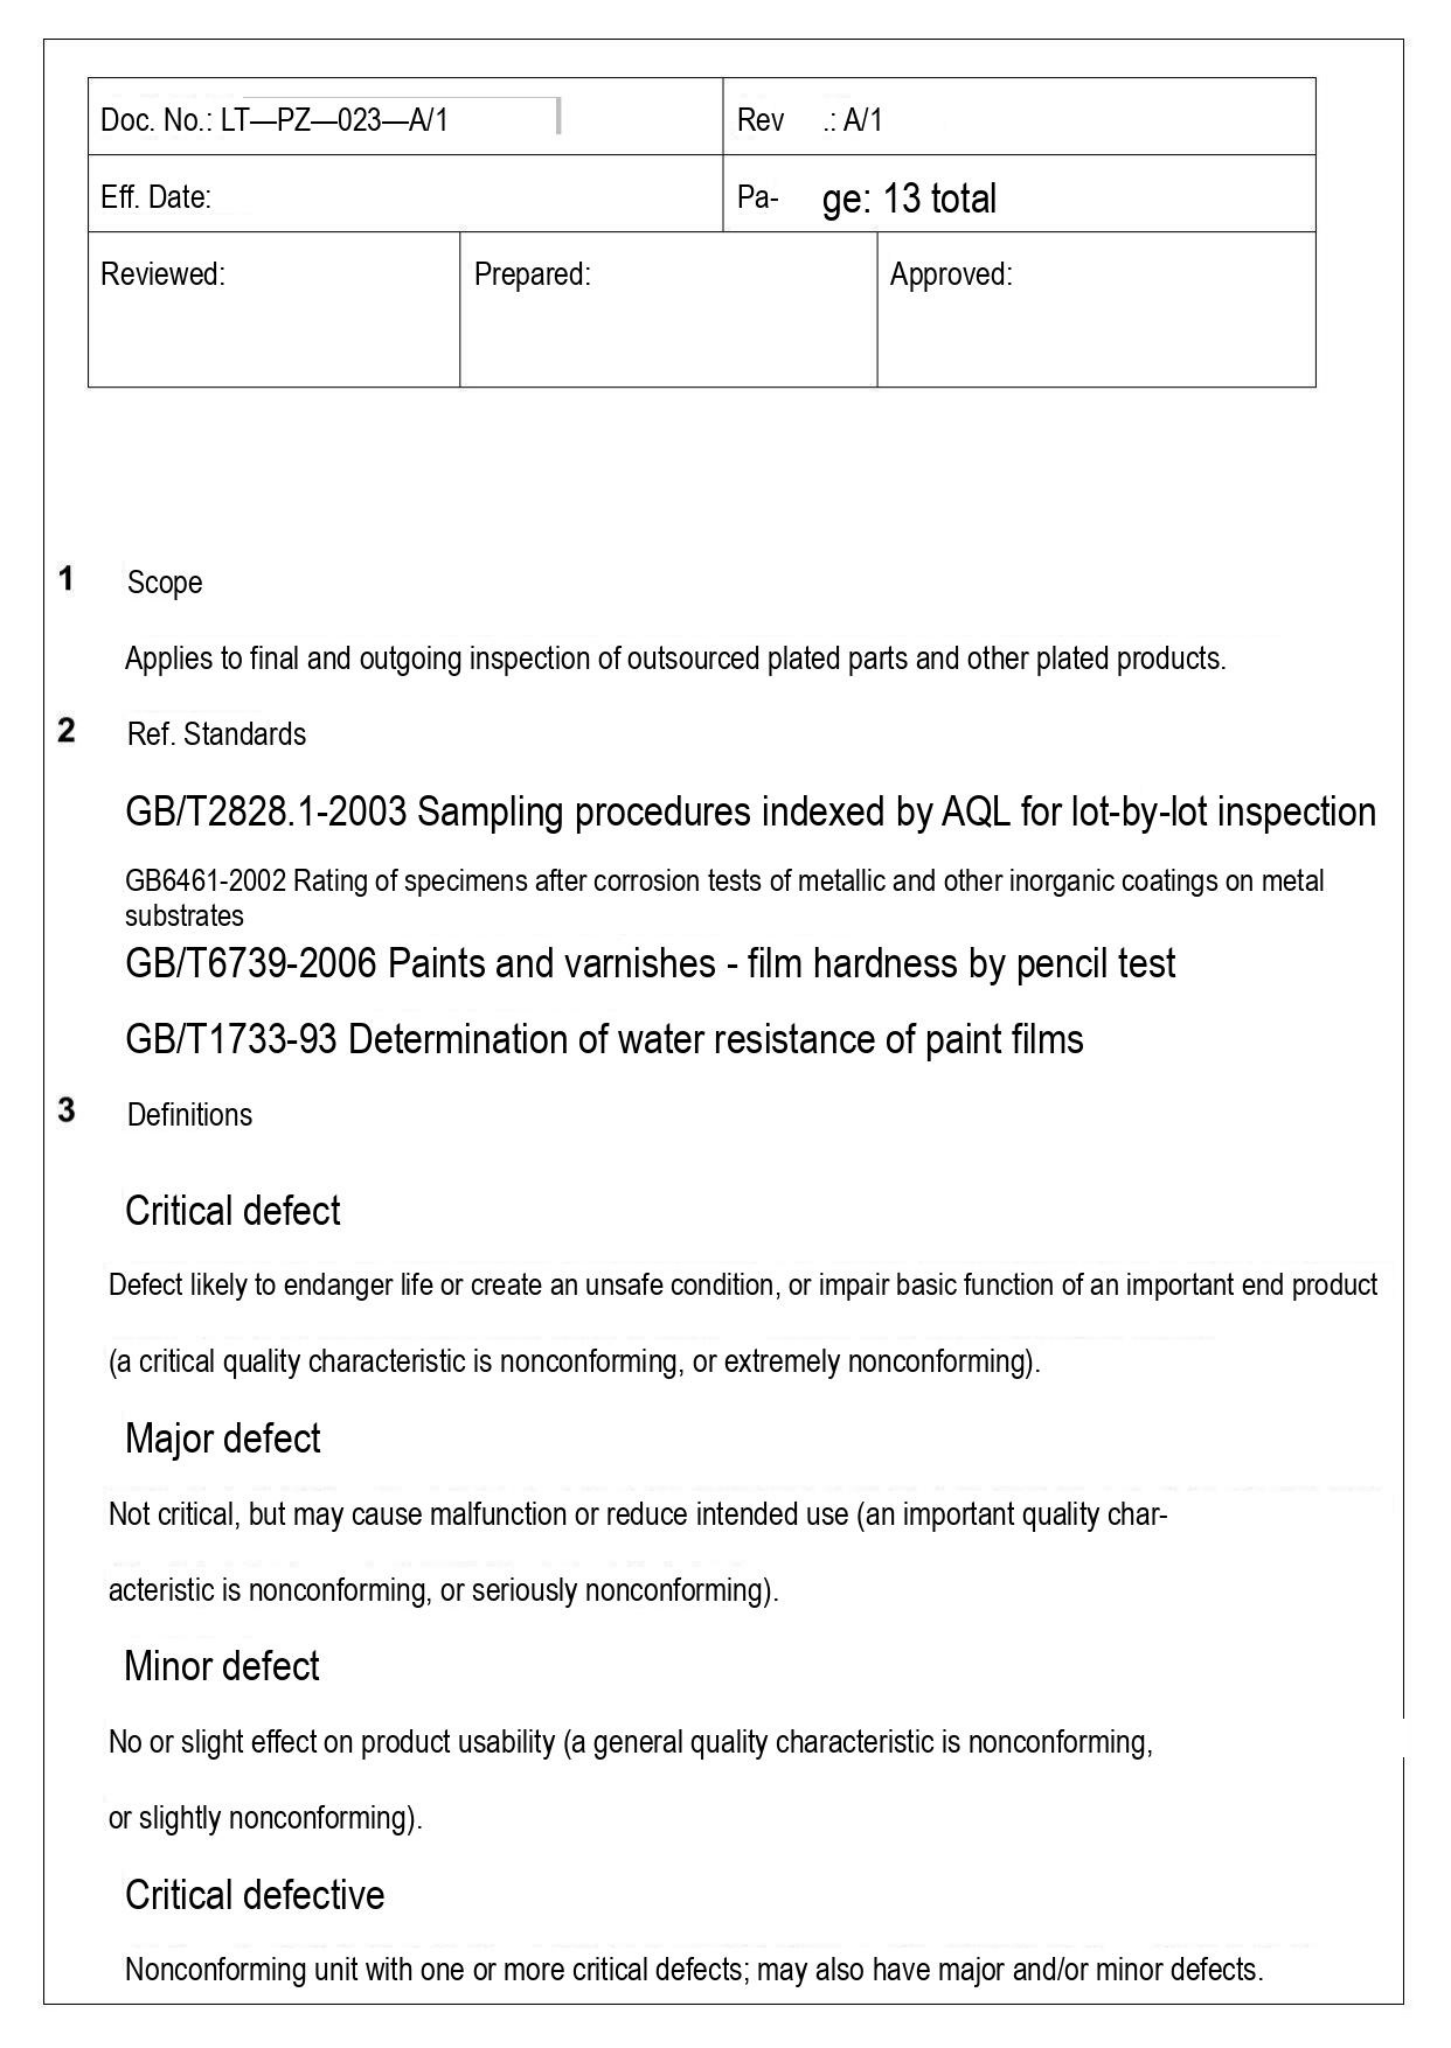| Doc. No.: LT—PZ—023—A/1 | | Rev .: A/1 |
|---|---|---|
| Eff. Date: | | Pa- ge: 13 total |
| Reviewed: | Prepared: | Approved: |

1 Scope

Applies to final and outgoing inspection of outsourced plated parts and other plated products.

2 Ref. Standards

GB/T2828.1-2003 Sampling procedures indexed by AQL for lot-by-lot inspection

GB6461-2002 Rating of specimens after corrosion tests of metallic and other inorganic coatings on metal substrates

GB/T6739-2006 Paints and varnishes - film hardness by pencil test

GB/T1733-93 Determination of water resistance of paint films

3 Definitions

Critical defect

Defect likely to endanger life or create an unsafe condition, or impair basic function of an important end product

(a critical quality characteristic is nonconforming, or extremely nonconforming).

Major defect

Not critical, but may cause malfunction or reduce intended use (an important quality char-

acteristic is nonconforming, or seriously nonconforming).

Minor defect

No or slight effect on product usability (a general quality characteristic is nonconforming,

or slightly nonconforming).

Critical defective

Nonconforming unit with one or more critical defects; may also have major and/or minor defects.
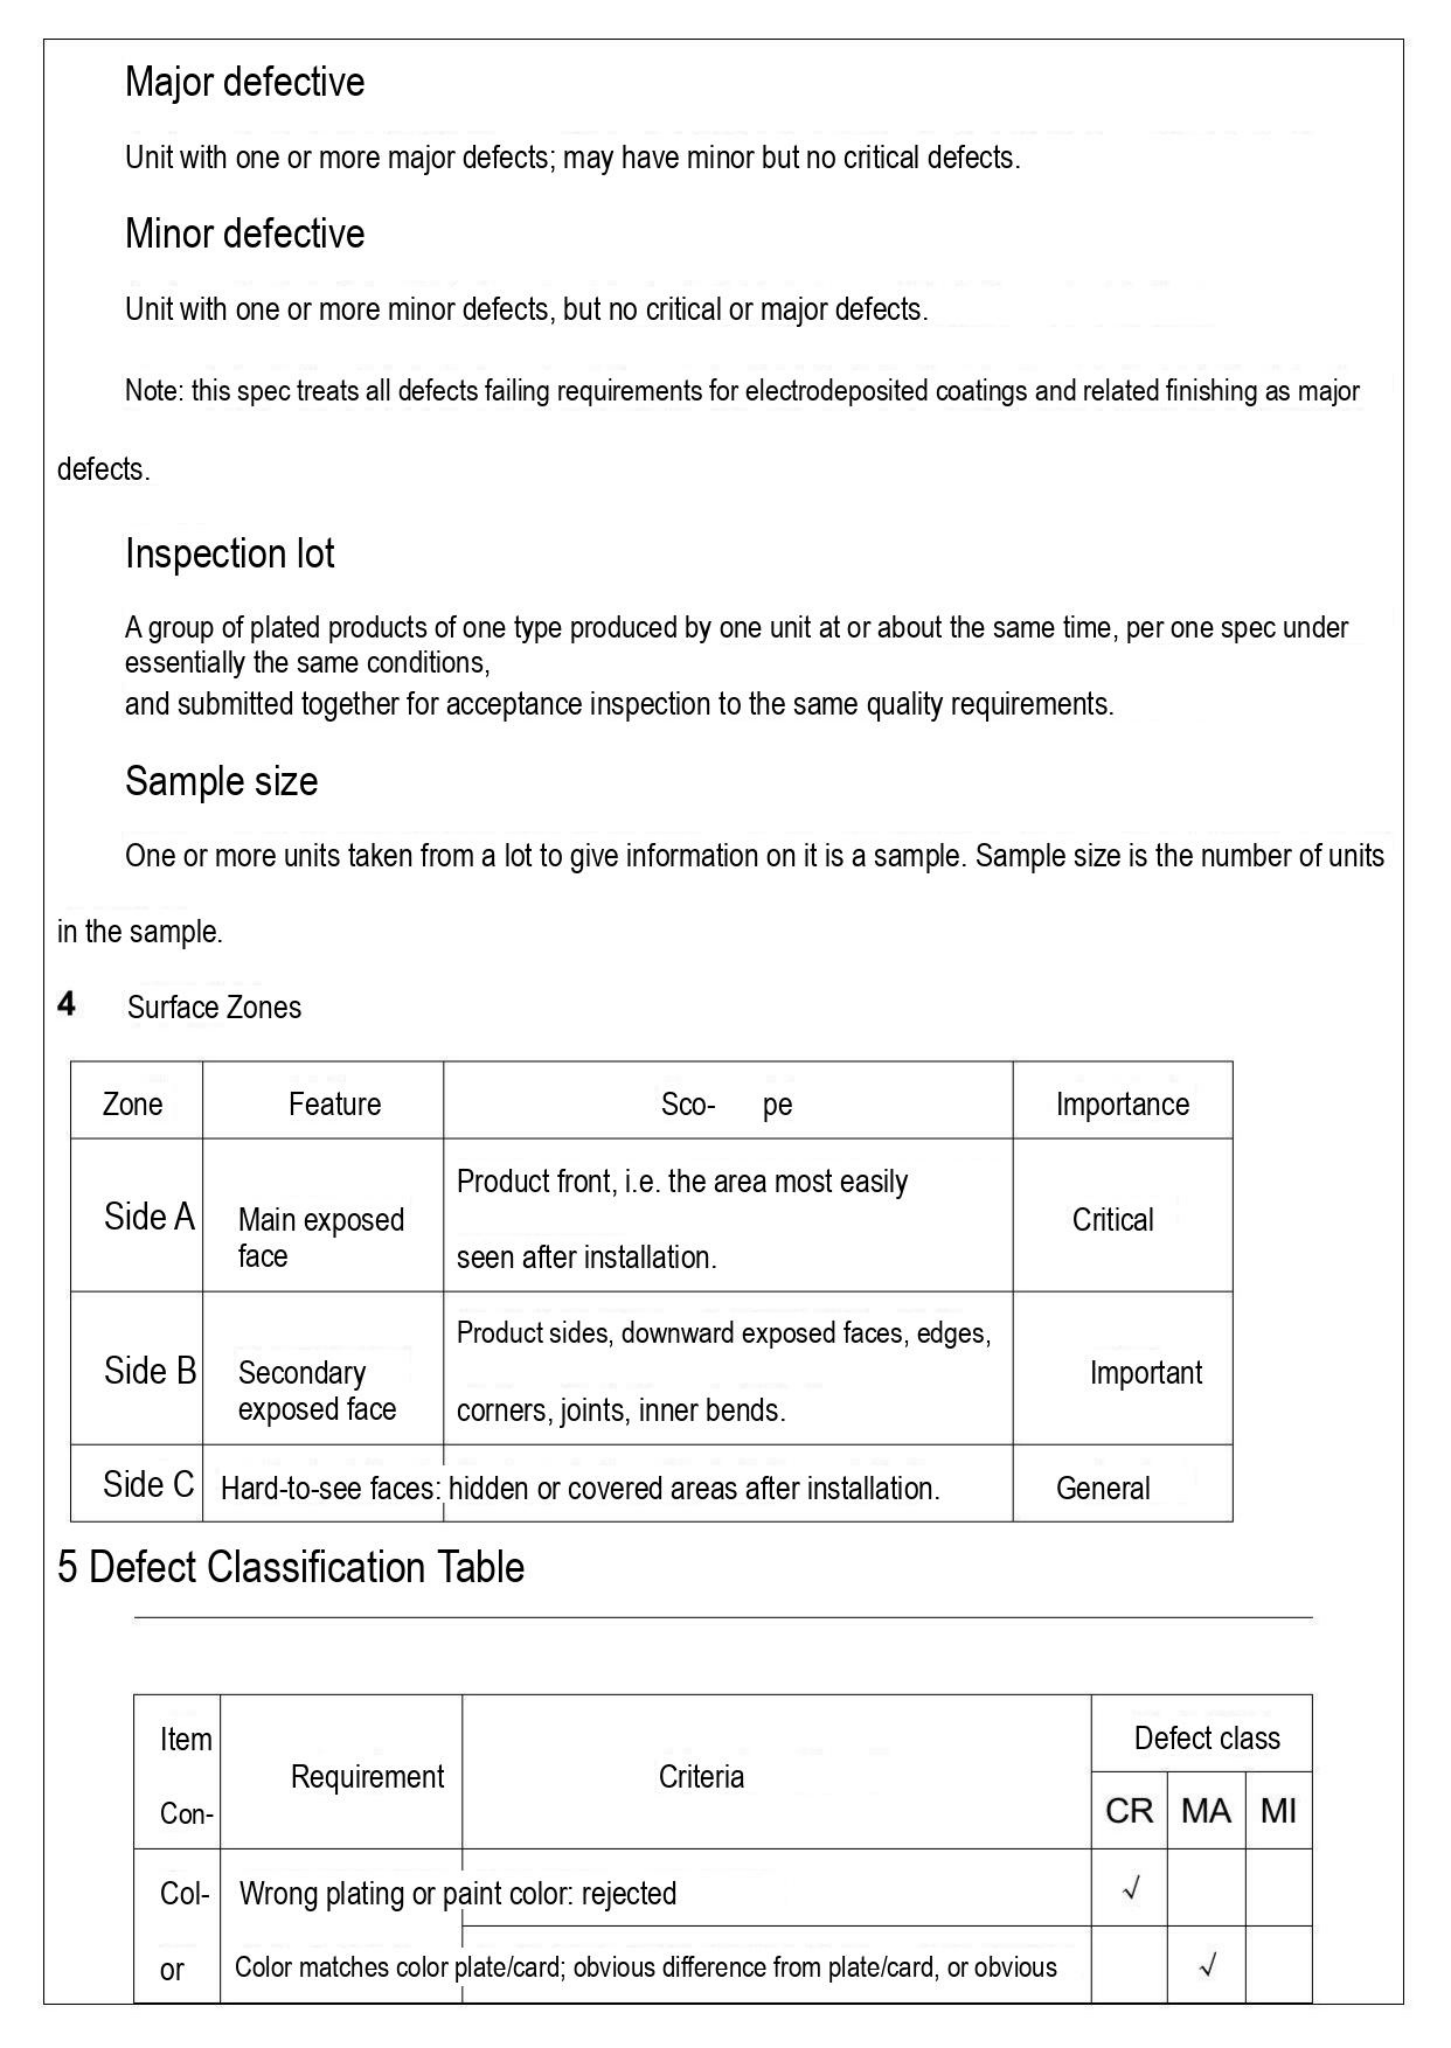Major defective

Unit with one or more major defects; may have minor but no critical defects.

Minor defective

Unit with one or more minor defects, but no critical or major defects.

Note: this spec treats all defects failing requirements for electrodeposited coatings and related finishing as major defects.

Inspection lot

A group of plated products of one type produced by one unit at or about the same time, per one spec under essentially the same conditions,
and submitted together for acceptance inspection to the same quality requirements.

Sample size

One or more units taken from a lot to give information on it is a sample. Sample size is the number of units in the sample.

4 Surface Zones

| Zone | Feature | Sco- pe | Importance |
|---|---|---|---|
| Side A | Main exposed face | Product front, i.e. the area most easily seen after installation. | Critical |
| Side B | Secondary exposed face | Product sides, downward exposed faces, edges, corners, joints, inner bends. | Important |
| Side C | Hard-to-see faces: hidden or covered areas after installation. | | General |

5 Defect Classification Table

| Item Con- | Requirement | Criteria | Defect class CR | Defect class MA | Defect class MI |
|---|---|---|---|---|---|
| Col- or | Wrong plating or paint color: rejected | | √ | | |
| | Color matches color plate/card; obvious difference from plate/card, or obvious | | | √ | |
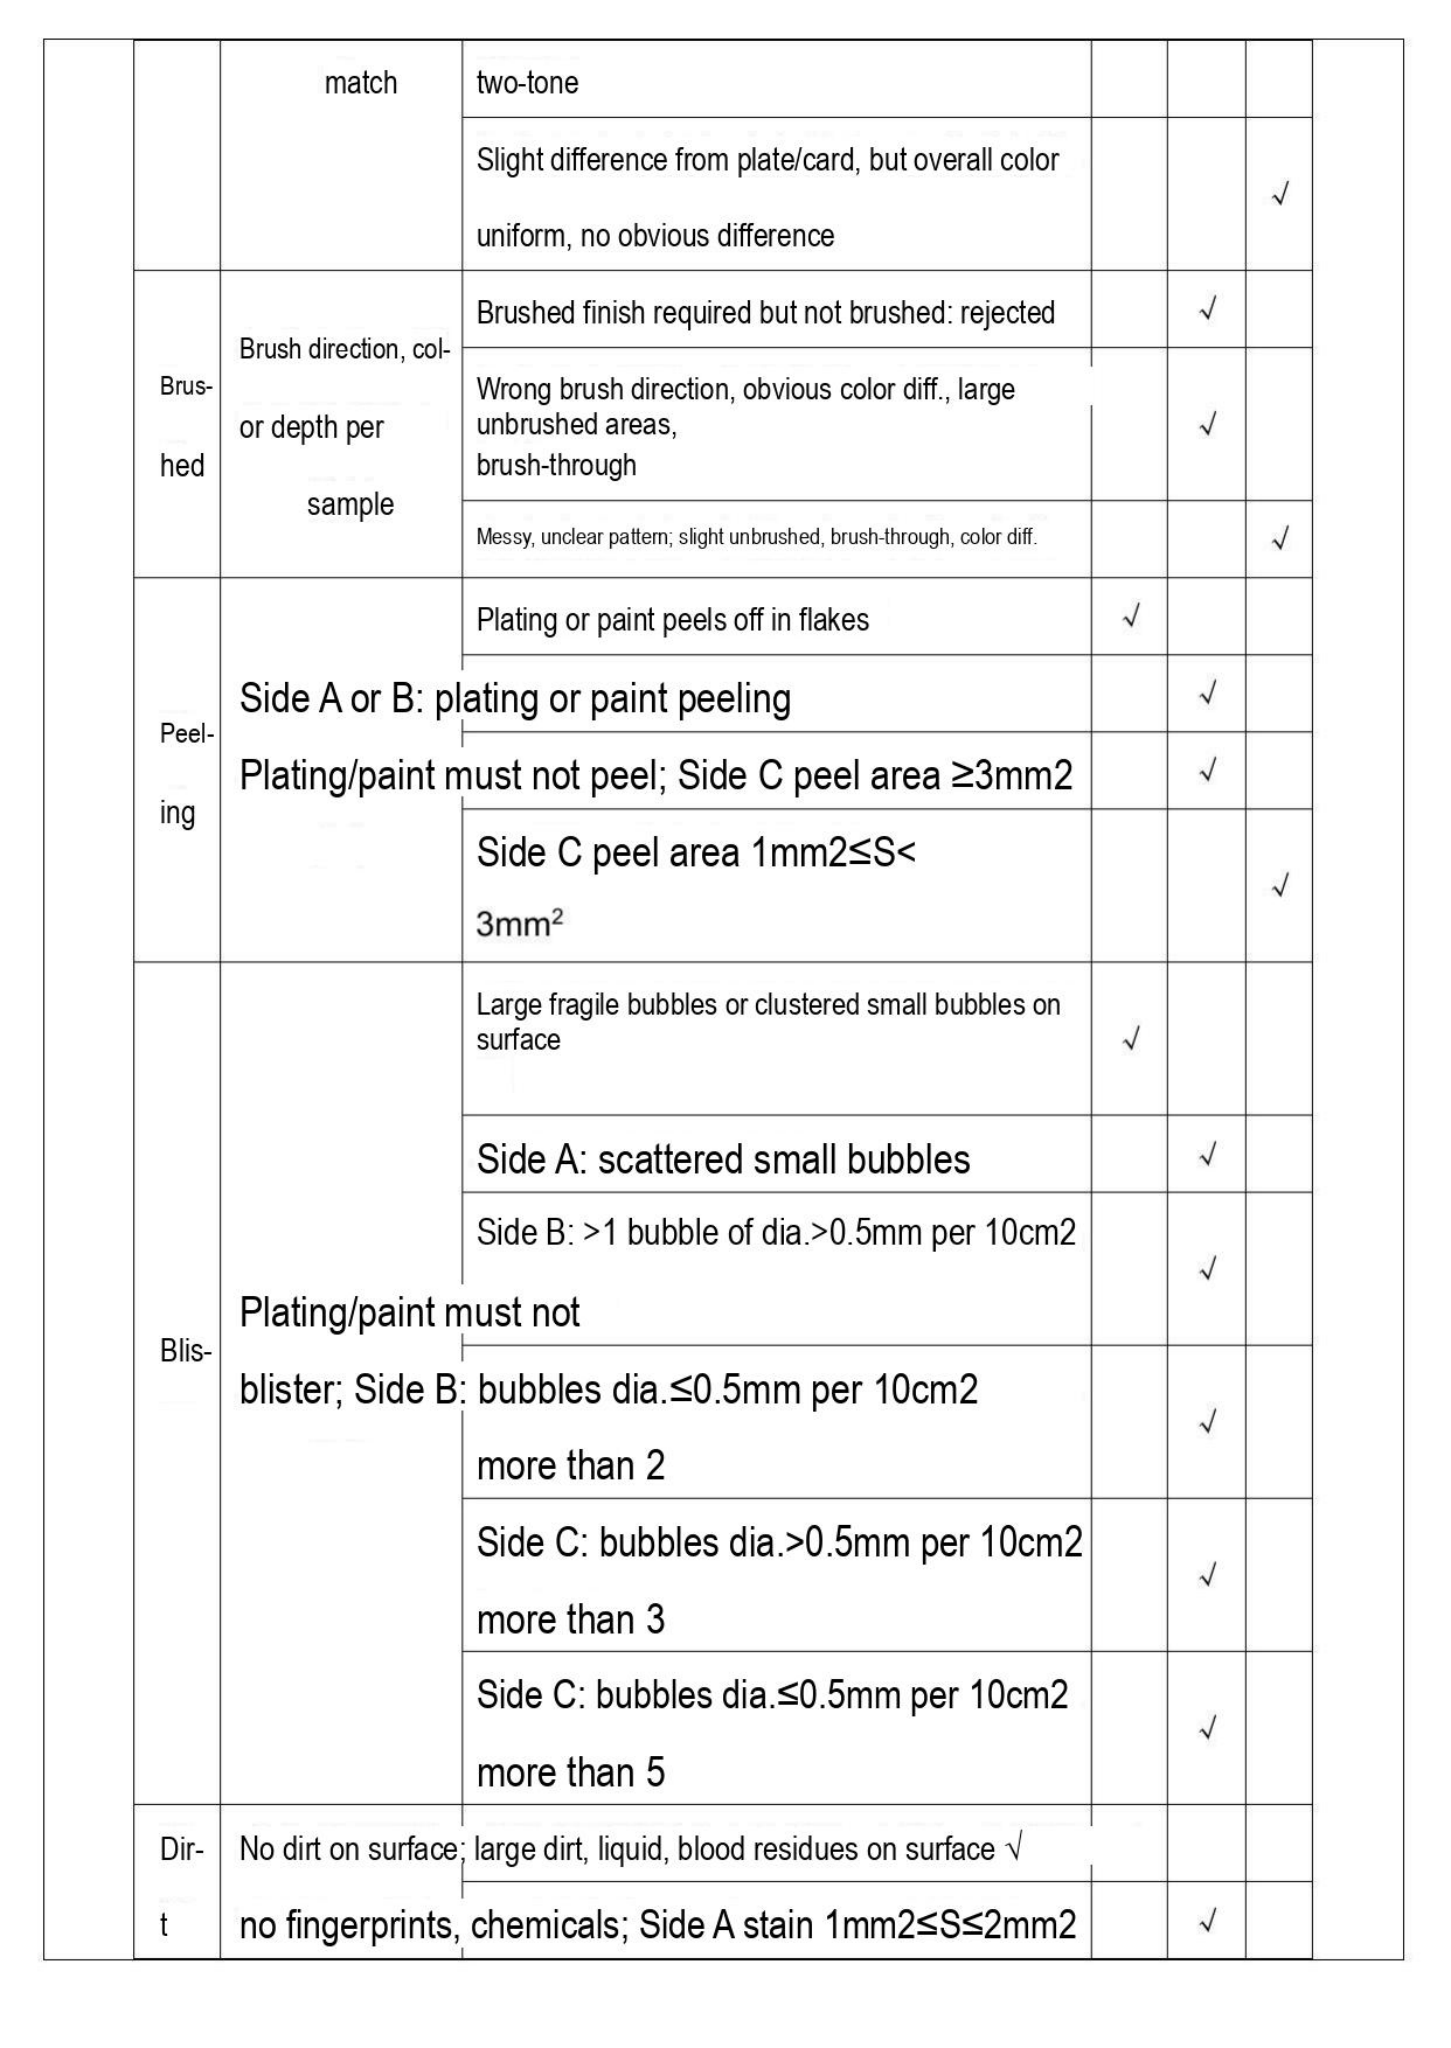| | | | | | | | |
|---|---|---|---|---|---|---|---|
| | | match | two-tone | | | | |
| | | | Slight difference from plate/card, but overall color uniform, no obvious difference | | | √ | |
| | Brus- hed | Brush direction, col- or depth per sample | Brushed finish required but not brushed: rejected | | √ | | |
| | | | Wrong brush direction, obvious color diff., large unbrushed areas, brush-through | | √ | | |
| | | | Messy, unclear pattern; slight unbrushed, brush-through, color diff. | | | √ | |
| | Peel- ing | | Plating or paint peels off in flakes | √ | | | |
| | | | Side A or B: plating or paint peeling | | √ | | |
| | | Plating/paint must not peel; | Side C peel area ≥3mm2 | | √ | | |
| | | | Side C peel area 1mm2≤S< 3mm² | | | √ | |
| | Blis- | | Large fragile bubbles or clustered small bubbles on surface | √ | | | |
| | | | Side A: scattered small bubbles | | √ | | |
| | | | Side B: >1 bubble of dia.>0.5mm per 10cm2 | | √ | | |
| | | Plating/paint must not blister; | Side B: bubbles dia.≤0.5mm per 10cm2 more than 2 | | √ | | |
| | | | Side C: bubbles dia.>0.5mm per 10cm2 more than 3 | | √ | | |
| | | | Side C: bubbles dia.≤0.5mm per 10cm2 more than 5 | | √ | | |
| | Dir- t | No dirt on surface; | large dirt, liquid, blood residues on surface √ | | | | |
| | | no fingerprints, chemicals; | Side A stain 1mm2≤S≤2mm2 | | √ | | |
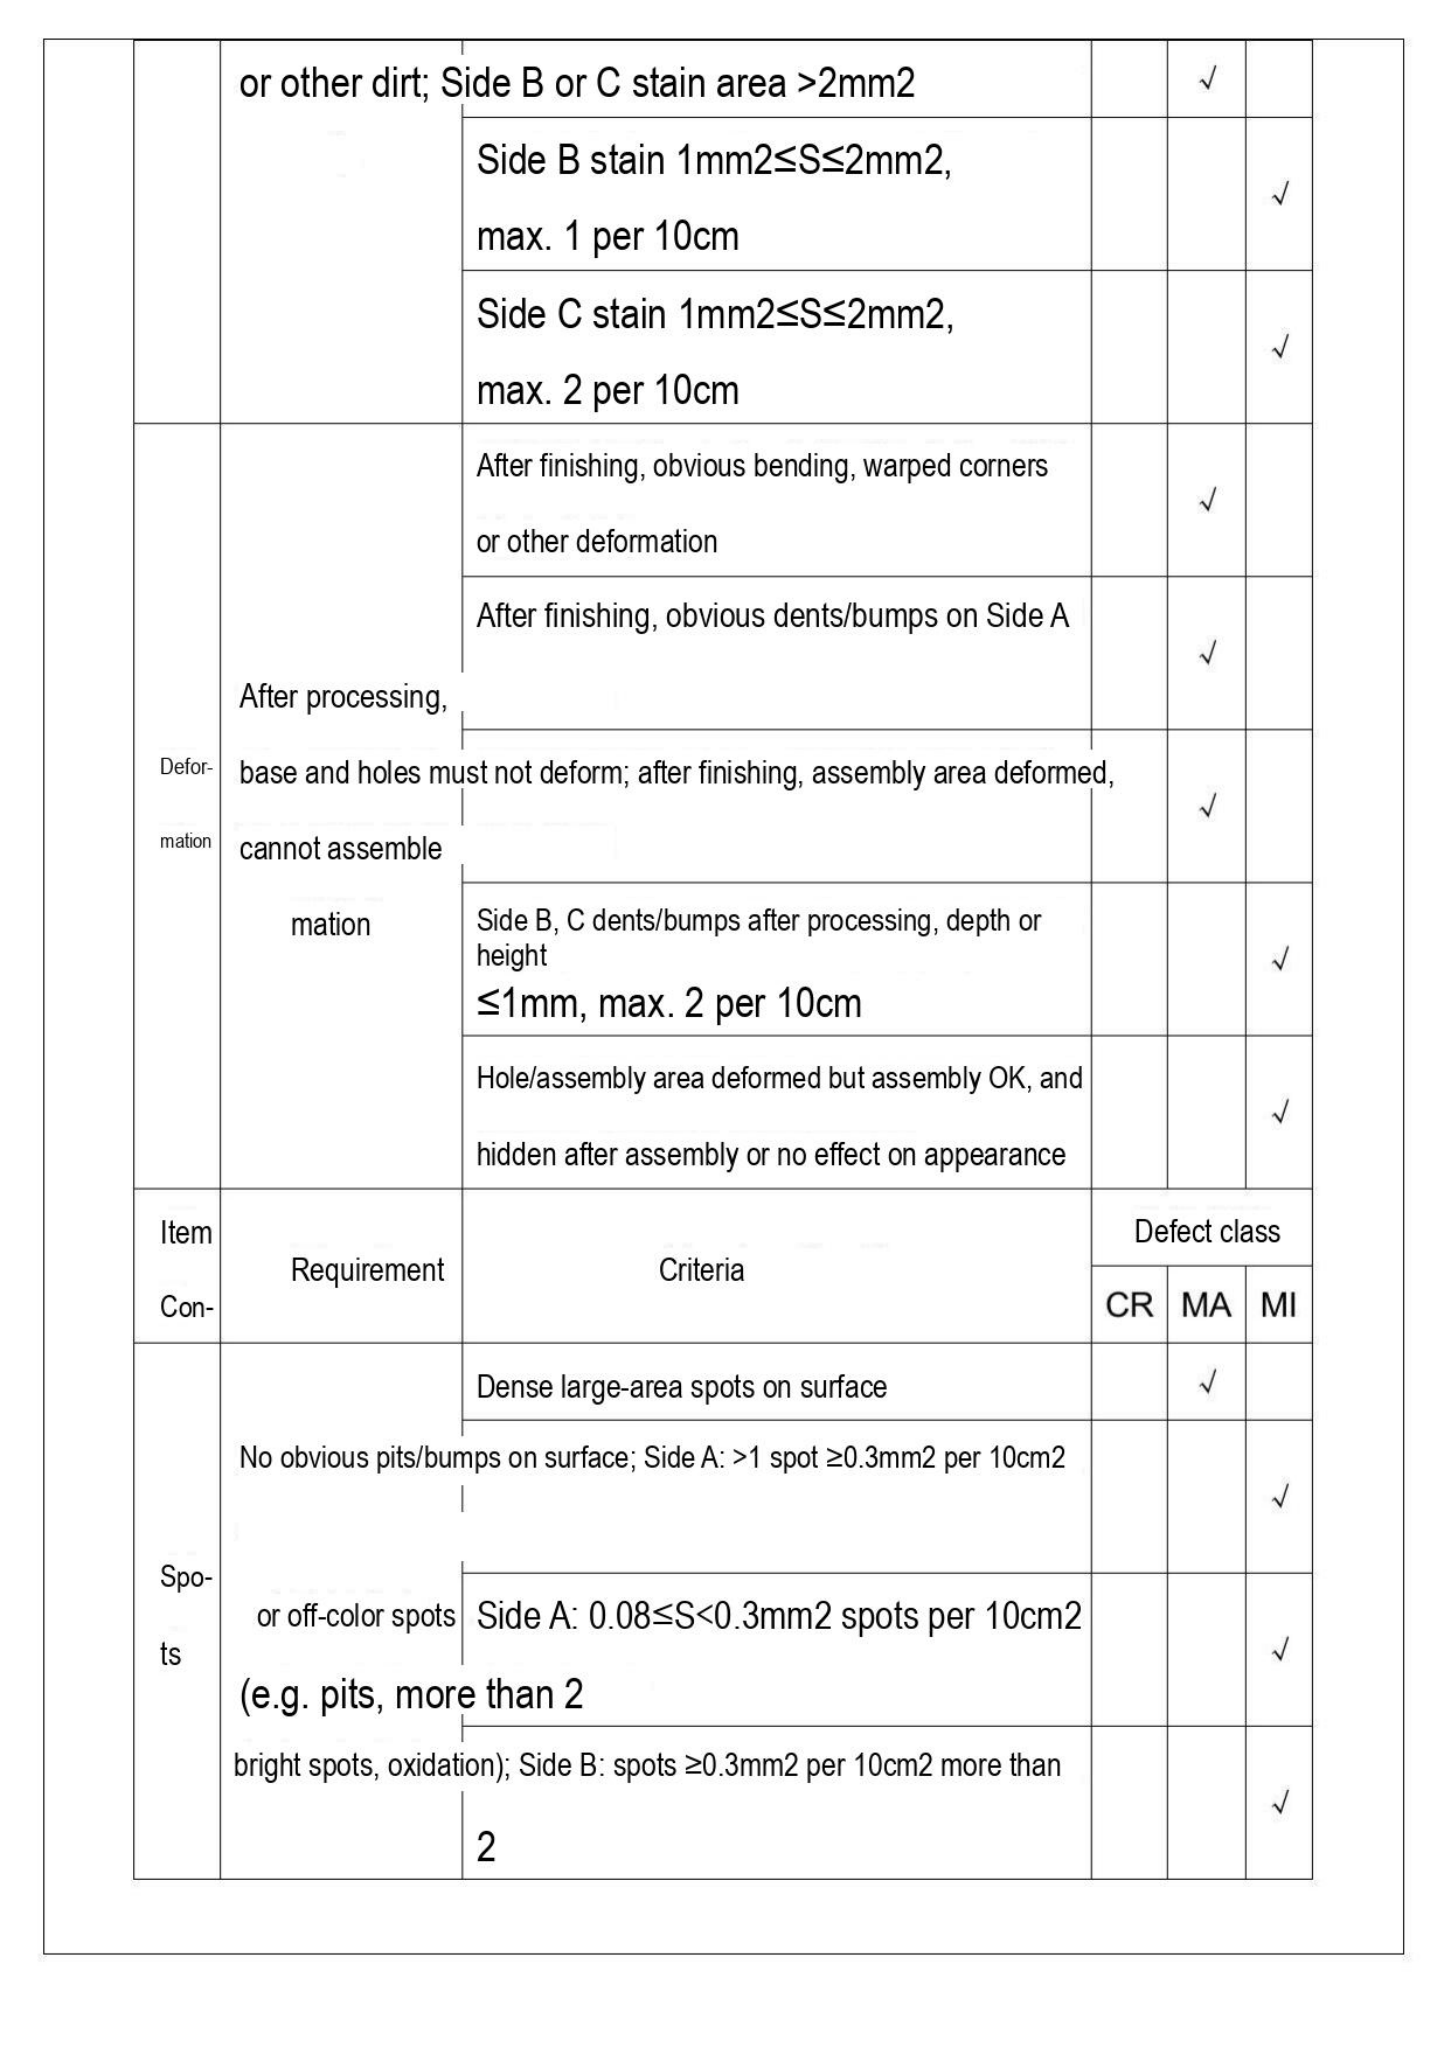| | | | | | |
|---|---|---|---|---|---|
| | or other dirt; Side B or C stain area >2mm2 | | | √ | |
| | | Side B stain 1mm2≤S≤2mm2, max. 1 per 10cm | | | √ |
| | | Side C stain 1mm2≤S≤2mm2, max. 2 per 10cm | | | √ |
| Defor- mation | | After finishing, obvious bending, warped corners or other deformation | | √ | |
| | | After finishing, obvious dents/bumps on Side A | | √ | |
| | After processing, base and holes must not deform; after finishing, assembly area deformed, cannot assemble | | | √ | |
| | mation | Side B, C dents/bumps after processing, depth or height ≤1mm, max. 2 per 10cm | | | √ |
| | | Hole/assembly area deformed but assembly OK, and hidden after assembly or no effect on appearance | | | √ |

| Item Con- | Requirement | Criteria | Defect class CR | Defect class MA | Defect class MI |
|---|---|---|---|---|---|
| Spo- ts | | Dense large-area spots on surface | | √ | |
| | No obvious pits/bumps on surface; Side A: >1 spot ≥0.3mm2 per 10cm2 | | | | √ |
| | or off-color spots (e.g. pits, more than 2 | Side A: 0.08≤S<0.3mm2 spots per 10cm2 | | | √ |
| | bright spots, oxidation); Side B: spots ≥0.3mm2 per 10cm2 more than 2 | | | | √ |
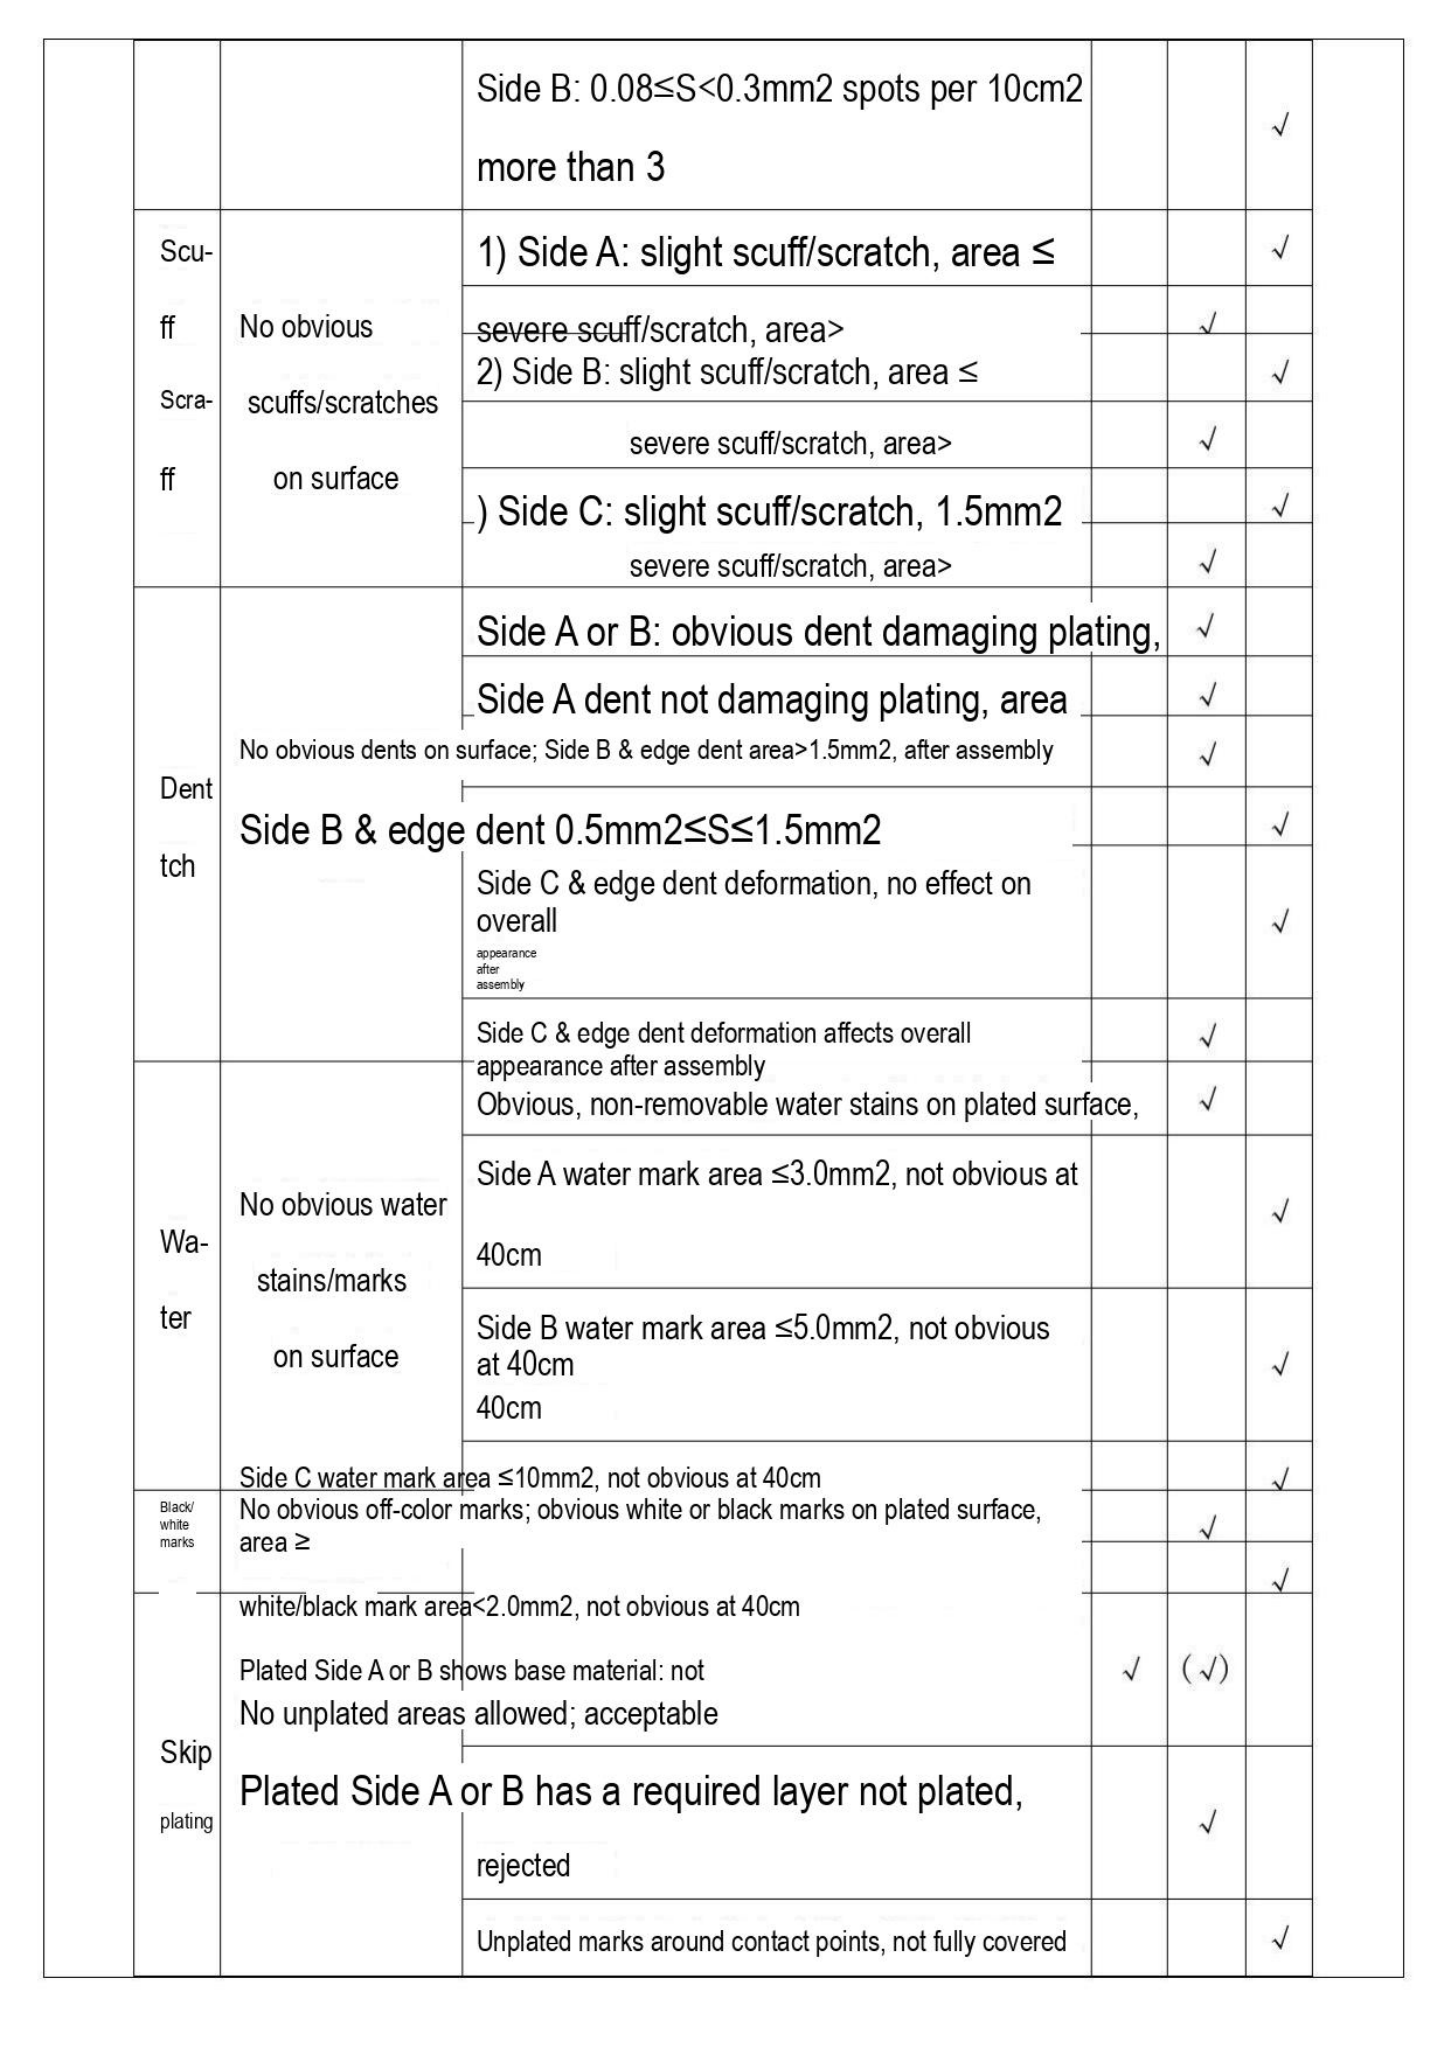|  |  |  |  |  |  |
|---|---|---|---|---|---|
|  |  | Side B: 0.08≤S<0.3mm2 spots per 10cm2 more than 3 |  |  | √ |
| Scu-ff Scra-ff | No obvious scuffs/scratches on surface | 1) Side A: slight scuff/scratch, area ≤ |  |  | √ |
|  |  | severe scuff/scratch, area> |  | √ |  |
|  |  | 2) Side B: slight scuff/scratch, area ≤ |  |  | √ |
|  |  | severe scuff/scratch, area> |  | √ |  |
|  |  | ) Side C: slight scuff/scratch, 1.5mm2 |  |  | √ |
|  |  | severe scuff/scratch, area> |  | √ |  |
| Dent tch | No obvious dents on surface; | Side A or B: obvious dent damaging plating, |  | √ |  |
|  |  | Side A dent not damaging plating, area |  | √ |  |
|  |  | Side B & edge dent area>1.5mm2, after assembly |  | √ |  |
|  |  | Side B & edge dent 0.5mm2≤S≤1.5mm2 |  |  | √ |
|  |  | Side C & edge dent deformation, no effect on overall appearance after assembly |  |  | √ |
|  |  | Side C & edge dent deformation affects overall appearance after assembly |  | √ |  |
| Wa-ter | No obvious water stains/marks on surface | Obvious, non-removable water stains on plated surface, |  | √ |  |
|  |  | Side A water mark area ≤3.0mm2, not obvious at 40cm |  |  | √ |
|  |  | Side B water mark area ≤5.0mm2, not obvious at 40cm 40cm |  |  | √ |
|  |  | Side C water mark area ≤10mm2, not obvious at 40cm |  |  | √ |
| Black/ white marks | No obvious off-color marks; | obvious white or black marks on plated surface, area ≥ |  | √ |  |
|  |  | white/black mark area<2.0mm2, not obvious at 40cm |  |  | √ |
| Skip plating | No unplated areas allowed; | Plated Side A or B shows base material: not acceptable | √ | (√) |  |
|  |  | Plated Side A or B has a required layer not plated, rejected |  | √ |  |
|  |  | Unplated marks around contact points, not fully covered |  |  | √ |
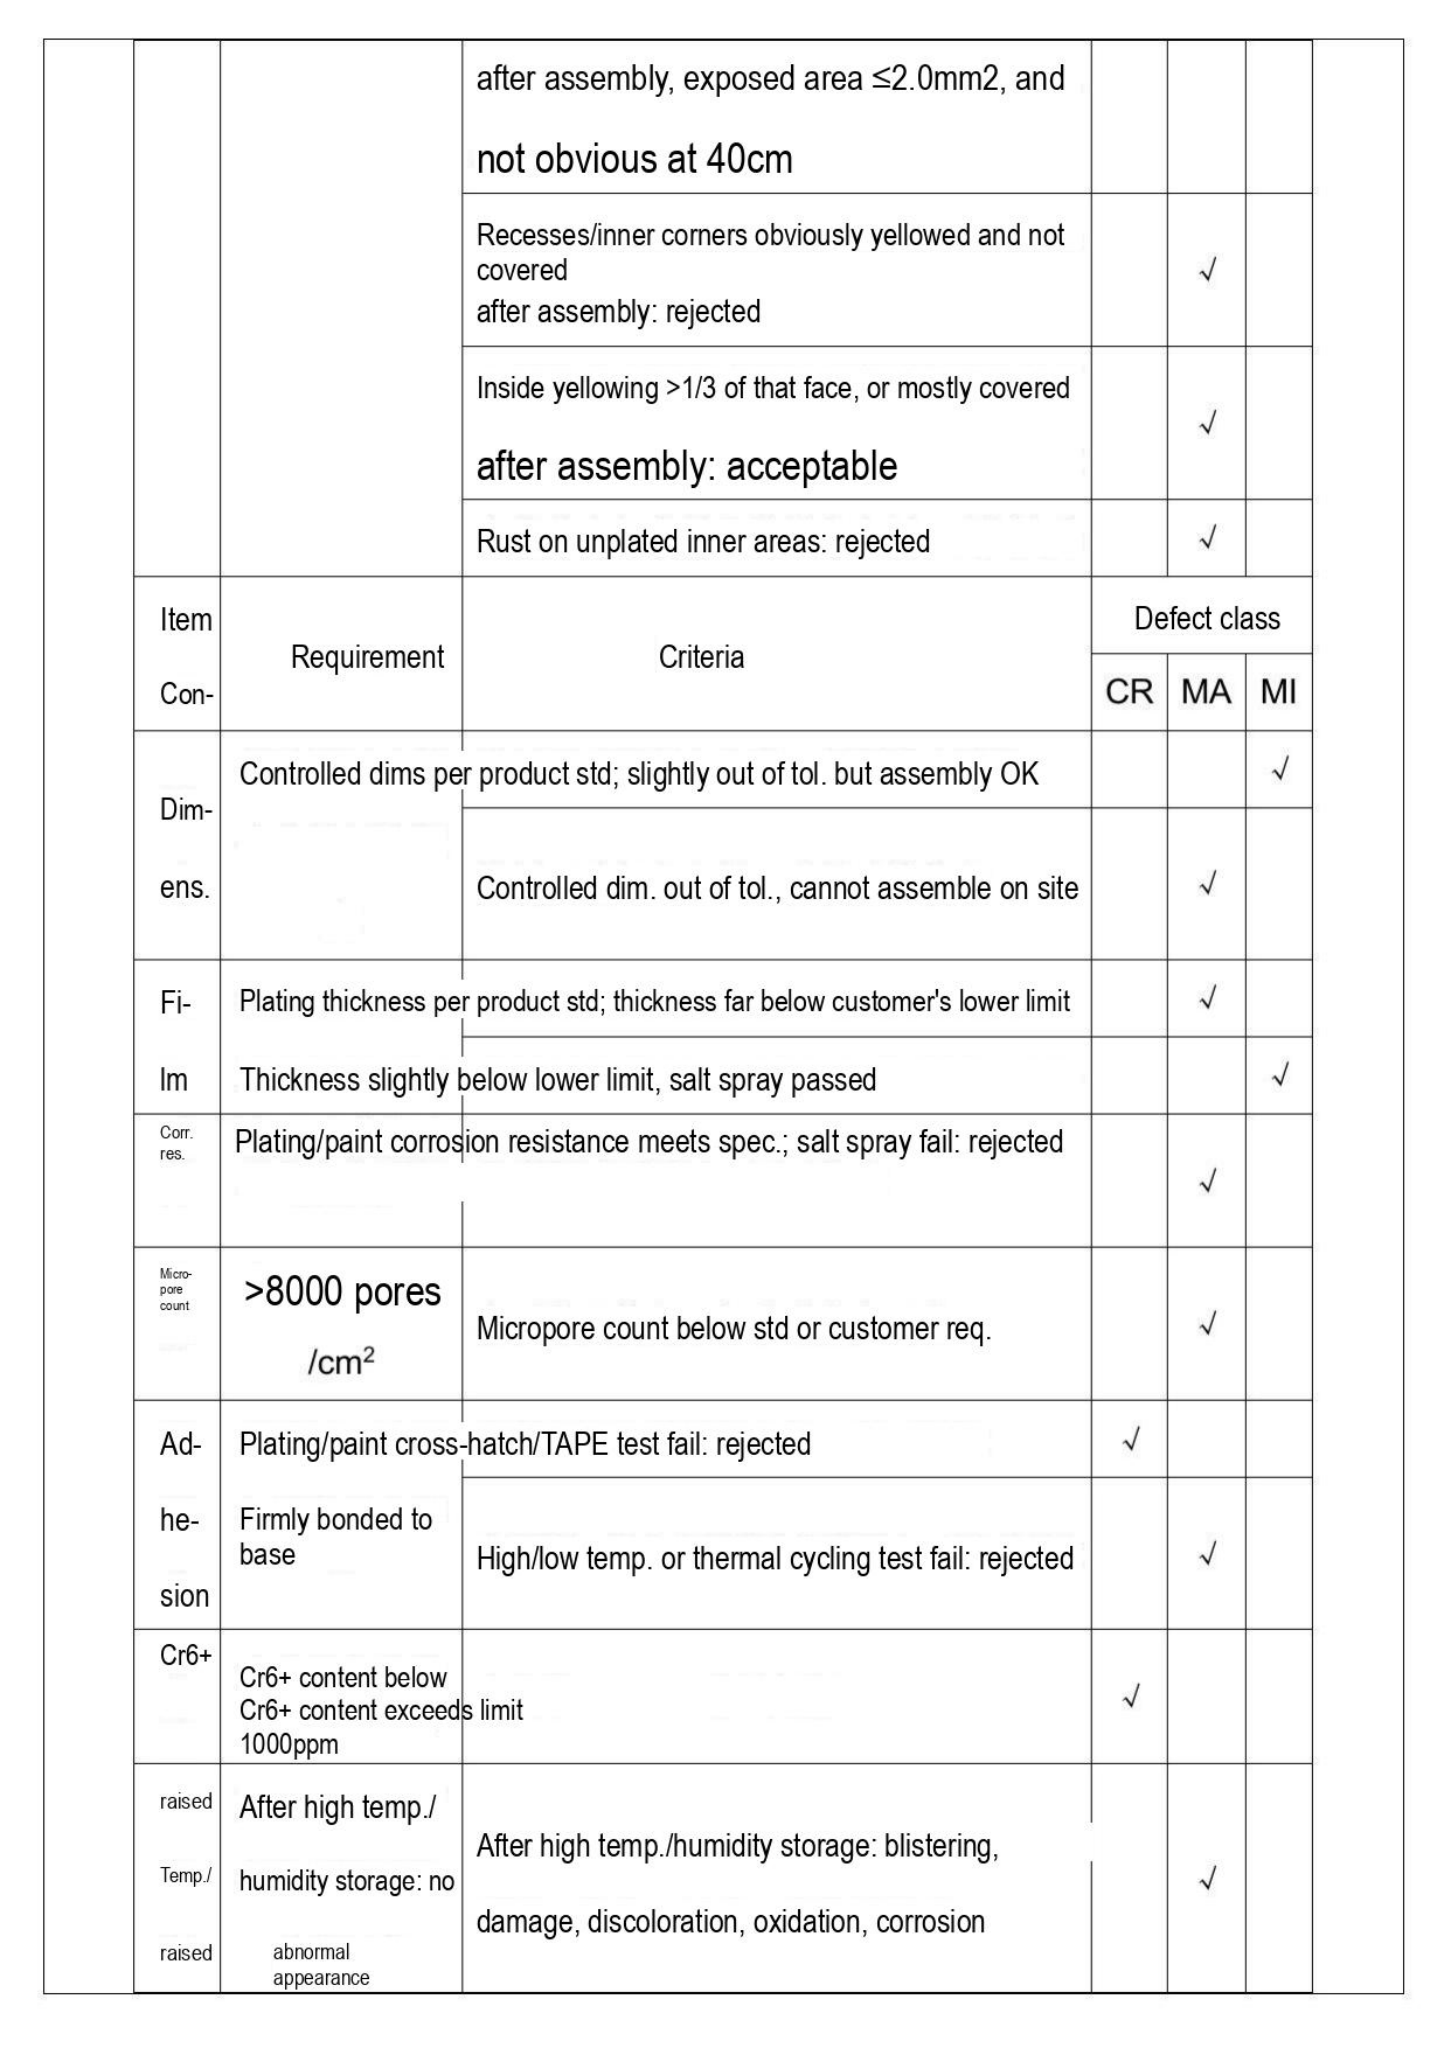| | | | | | |
|---|---|---|---|---|---|
| | | after assembly, exposed area ≤2.0mm2, and not obvious at 40cm | | | |
| | | Recesses/inner corners obviously yellowed and not covered after assembly: rejected | | √ | |
| | | Inside yellowing >1/3 of that face, or mostly covered after assembly: acceptable | | √ | |
| | | Rust on unplated inner areas: rejected | | √ | |

<table>
<tr><th rowspan="2">Item Con-</th><th rowspan="2">Requirement</th><th rowspan="2">Criteria</th><th colspan="3">Defect class</th></tr>
<tr><th>CR</th><th>MA</th><th>MI</th></tr>
<tr><td rowspan="2">Dim- ens.</td><td colspan="2">Controlled dims per product std; slightly out of tol. but assembly OK</td><td></td><td></td><td>√</td></tr>
<tr><td></td><td>Controlled dim. out of tol., cannot assemble on site</td><td></td><td>√</td><td></td></tr>
<tr><td rowspan="2">Fi- lm</td><td colspan="2">Plating thickness per product std; thickness far below customer's lower limit</td><td></td><td>√</td><td></td></tr>
<tr><td colspan="2">Thickness slightly below lower limit, salt spray passed</td><td></td><td></td><td>√</td></tr>
<tr><td>Corr. res.</td><td colspan="2">Plating/paint corrosion resistance meets spec.; salt spray fail: rejected</td><td></td><td>√</td><td></td></tr>
<tr><td>Micro-pore count</td><td>&gt;8000 pores /cm²</td><td>Micropore count below std or customer req.</td><td></td><td>√</td><td></td></tr>
<tr><td rowspan="2">Ad- he- sion</td><td colspan="2">Plating/paint cross-hatch/TAPE test fail: rejected</td><td>√</td><td></td><td></td></tr>
<tr><td>Firmly bonded to base</td><td>High/low temp. or thermal cycling test fail: rejected</td><td></td><td>√</td><td></td></tr>
<tr><td>Cr6+</td><td colspan="2">Cr6+ content below<br>Cr6+ content exceeds limit<br>1000ppm</td><td>√</td><td></td><td></td></tr>
<tr><td>raised Temp./ raised</td><td>After high temp./ humidity storage: no abnormal appearance</td><td>After high temp./humidity storage: blistering, damage, discoloration, oxidation, corrosion</td><td></td><td>√</td><td></td></tr>
</table>
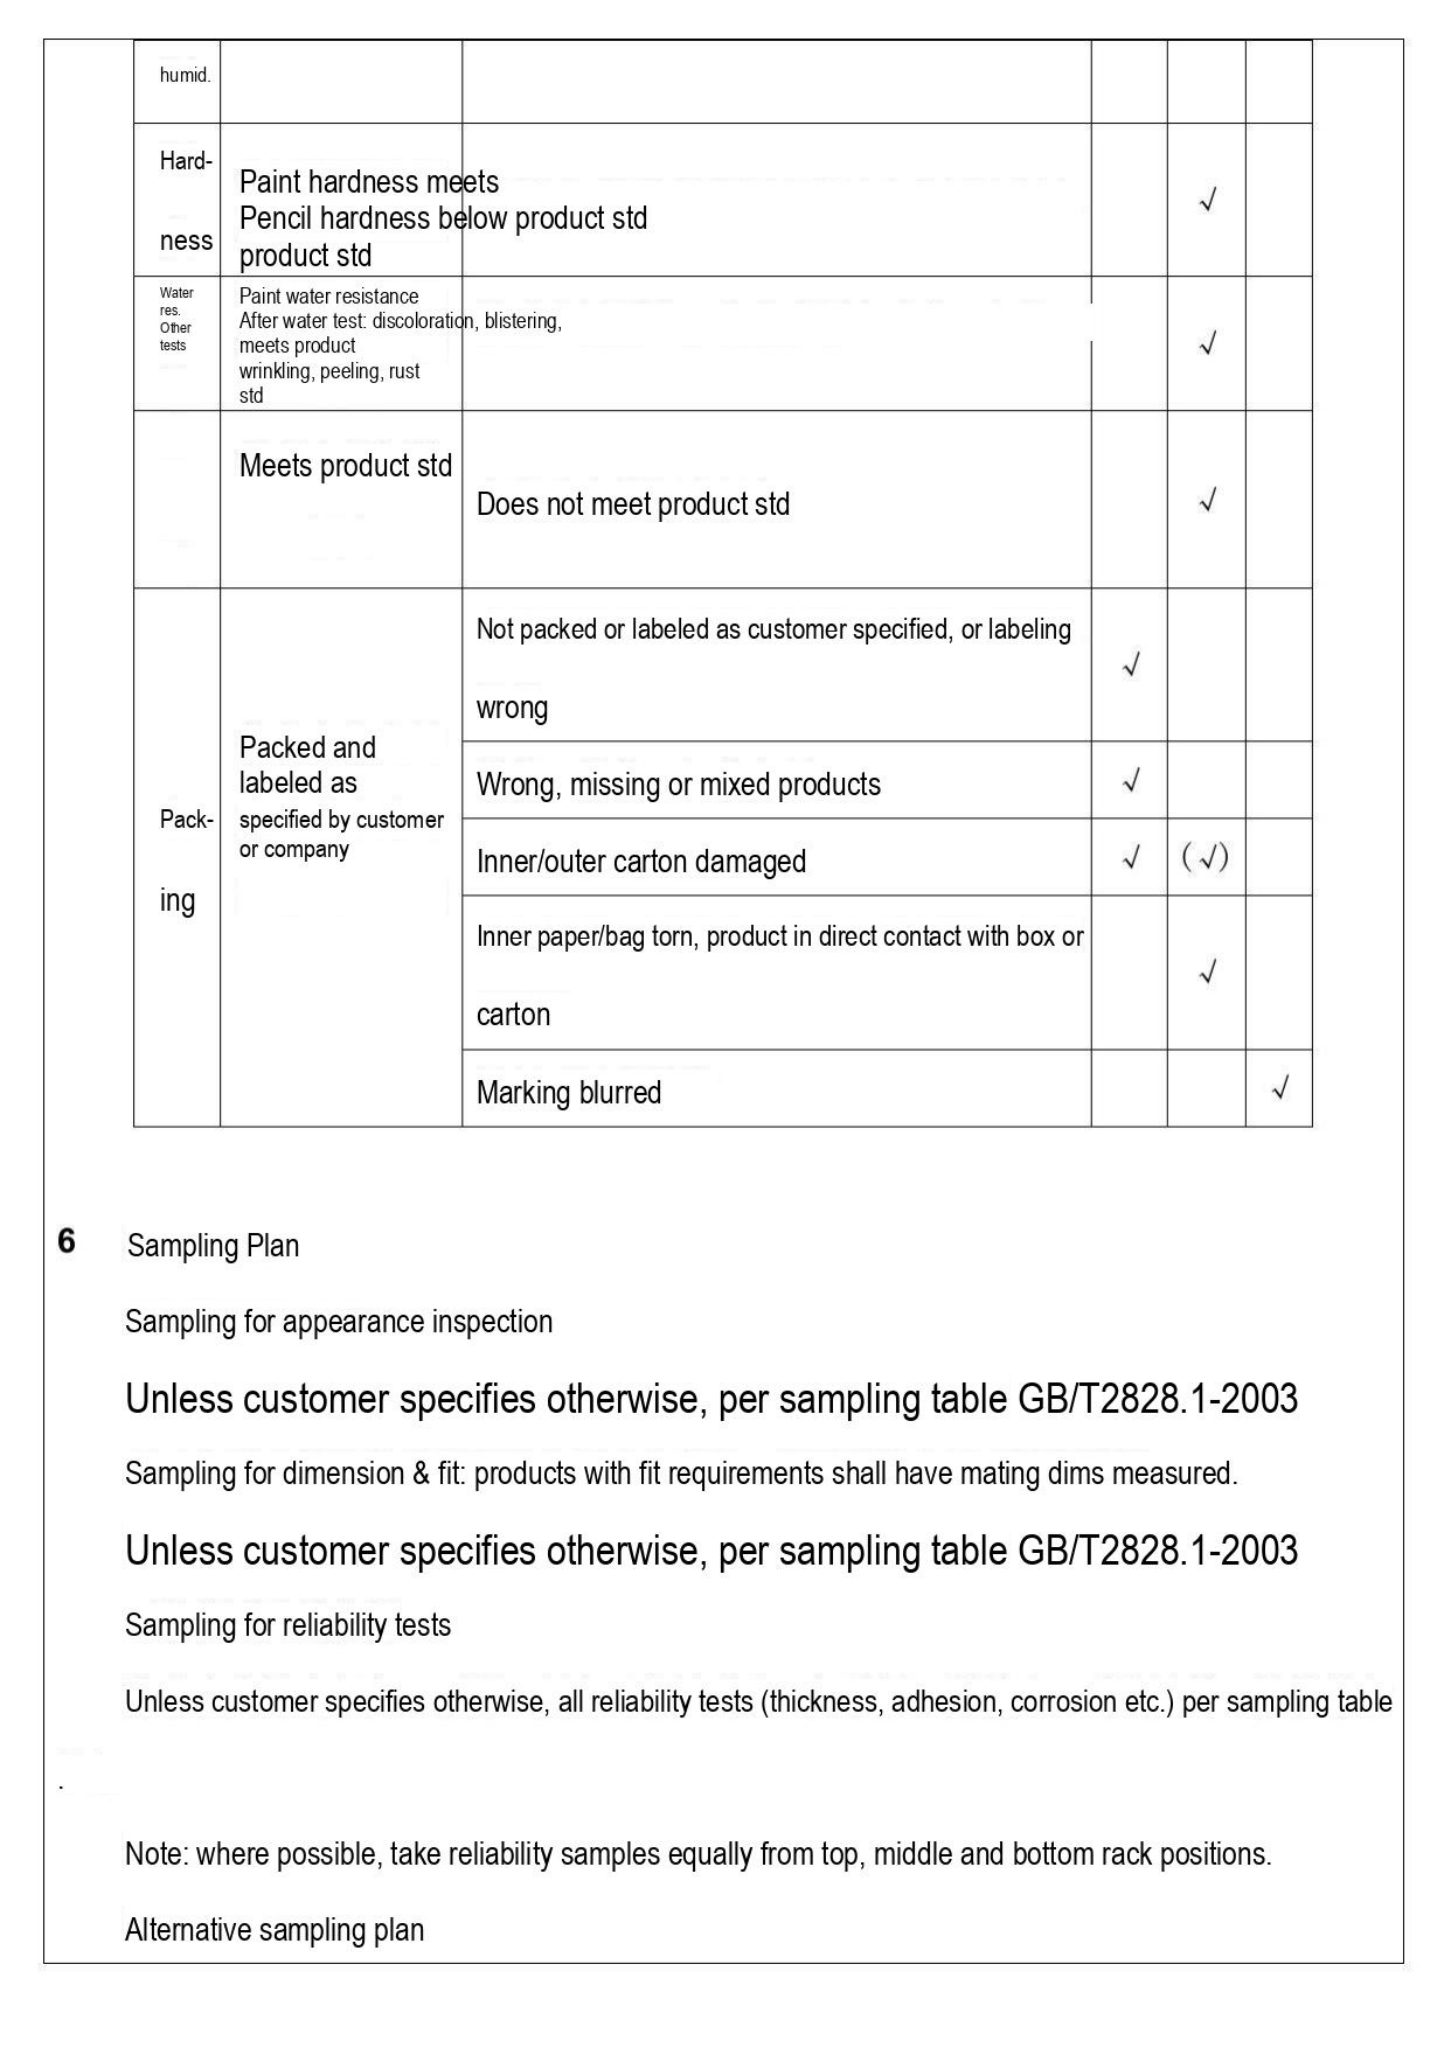| | | | | | |
|---|---|---|---|---|---|
| humid. | | | | | |
| Hard- ness | Paint hardness meets Pencil hardness below product std product std | | | √ | |
| Water res. Other tests | Paint water resistance After water test: discoloration, blistering, meets product wrinkling, peeling, rust std | | | √ | |
| | Meets product std | Does not meet product std | | √ | |
| Pack- ing | Packed and labeled as specified by customer or company | Not packed or labeled as customer specified, or labeling wrong | √ | | |
| | | Wrong, missing or mixed products | √ | | |
| | | Inner/outer carton damaged | √ | (√) | |
| | | Inner paper/bag torn, product in direct contact with box or carton | | √ | |
| | | Marking blurred | | | √ |

**6** Sampling Plan

Sampling for appearance inspection

Unless customer specifies otherwise, per sampling table GB/T2828.1-2003

Sampling for dimension & fit: products with fit requirements shall have mating dims measured.

Unless customer specifies otherwise, per sampling table GB/T2828.1-2003

Sampling for reliability tests

Unless customer specifies otherwise, all reliability tests (thickness, adhesion, corrosion etc.) per sampling table

Note: where possible, take reliability samples equally from top, middle and bottom rack positions.

Alternative sampling plan